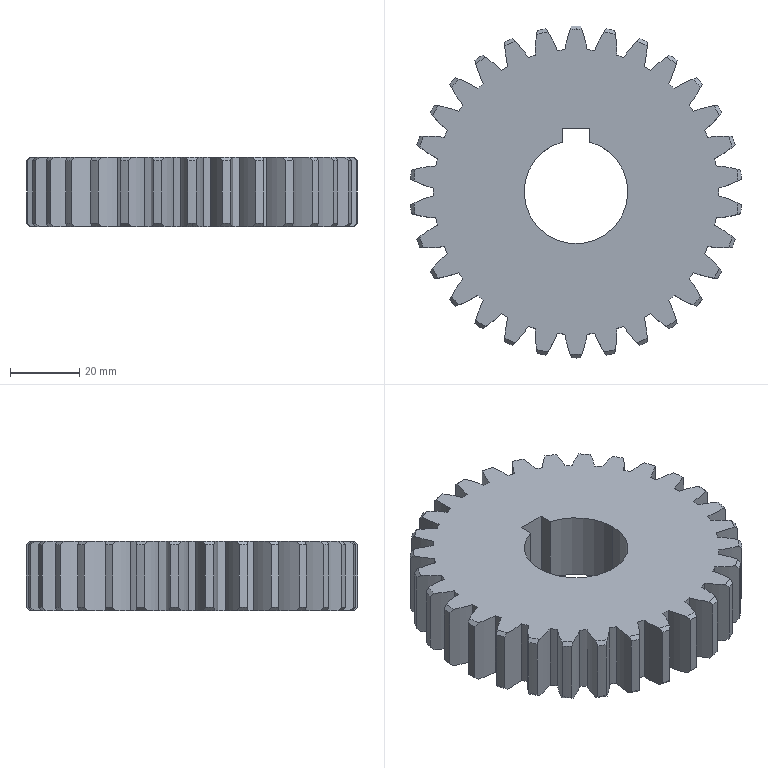Part | SolidWorks | features BaseBody 1 | 1 solid | 205 faces | box 95.704 x 96 x 20 mm | volume 90599 mm3 | cylinder 126 | cone 68 | plane 7 | spline 4 | commonest cylinder face diameters 60.03 x62 82.5 x31 96 x30 30 x3